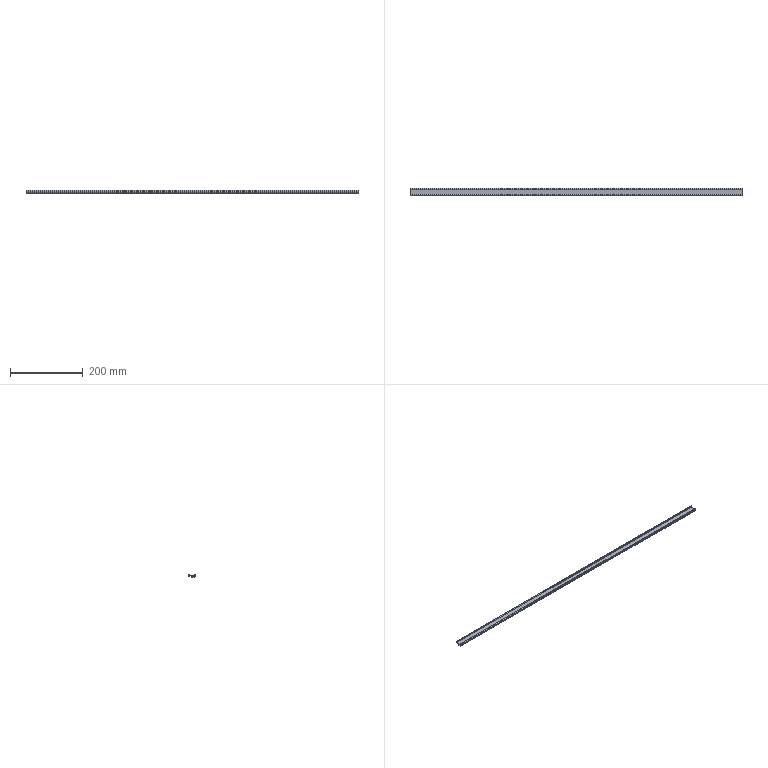Part | SolidWorks | features Extrusion 1 | 1 solid | 37 faces | box 915 x 19.991 x 9 mm | volume 36941 mm3 | cylinder 19 | plane 18 | commonest cylinder face diameters 2 x6 0.5 x5 0.2 x2 3 x2 4.958 x2 3.038 x1
STEP:
#1=CARTESIAN_POINT('',(492.5,771.135,454.913));
#2=VERTEX_POINT('',#1);
#3=CARTESIAN_POINT('',(492.5,769.976,455.201));
#4=VERTEX_POINT('',#3);
#5=CARTESIAN_POINT('',(492.5,769.976,452.722));
#6=DIRECTION('',(1.,0.,0.));
#7=DIRECTION('',(0.,0.,-1.));
#8=AXIS2_PLACEMENT_3D('',#5,#6,#7);
#9=CIRCLE('',#8,2.479);
#10=EDGE_CURVE('',#2,#4,#9,.T.);
#11=ORIENTED_EDGE('',*,*,#10,.T.);
#12=CARTESIAN_POINT('',(-422.5,769.976,455.201));
#13=VERTEX_POINT('',#12);
#14=CARTESIAN_POINT('',(492.5,769.976,455.201));
#15=DIRECTION('',(-1.,0.,0.));
#16=VECTOR('',#15,1000.);
#17=LINE('',#14,#16);
#18=EDGE_CURVE('',#4,#13,#17,.T.);
#19=ORIENTED_EDGE('',*,*,#18,.T.);
#20=CARTESIAN_POINT('',(-422.5,771.135,454.913));
#21=VERTEX_POINT('',#20);
#22=CARTESIAN_POINT('',(-422.5,769.976,452.722));
#23=DIRECTION('',(1.,0.,0.));
#24=DIRECTION('',(0.,0.,-1.));
#25=AXIS2_PLACEMENT_3D('',#22,#23,#24);
#26=CIRCLE('',#25,2.479);
#27=EDGE_CURVE('',#21,#13,#26,.T.);
#28=ORIENTED_EDGE('',*,*,#27,.F.);
#29=CARTESIAN_POINT('',(492.5,771.135,454.913));
#30=DIRECTION('',(-1.,0.,0.));
#31=VECTOR('',#30,1000.);
#32=LINE('',#29,#31);
#33=EDGE_CURVE('',#2,#21,#32,.T.);
#34=ORIENTED_EDGE('',*,*,#33,.F.);
#35=EDGE_LOOP('',(#11,#19,#28,#34));
#36=FACE_OUTER_BOUND('',#35,.T.);
#37=CARTESIAN_POINT('',(492.5,769.976,452.722));
#38=DIRECTION('',(-1.,0.,0.));
#39=DIRECTION('',(0.,0.,1.));
#40=AXIS2_PLACEMENT_3D('',#37,#38,#39);
#41=CYLINDRICAL_SURFACE('',#40,2.479);
#42=ADVANCED_FACE('',(#36),#41,.F.);
#43=CARTESIAN_POINT('',(-422.5,755.36,455.2));
#44=VERTEX_POINT('',#43);
#45=CARTESIAN_POINT('',(-422.5,755.11,454.95));
#46=VERTEX_POINT('',#45);
#47=CARTESIAN_POINT('',(-422.5,755.36,454.95));
#48=DIRECTION('',(1.,0.,0.));
#49=DIRECTION('',(0.,0.,-1.));
#50=AXIS2_PLACEMENT_3D('',#47,#48,#49);
#51=CIRCLE('',#50,0.25);
#52=EDGE_CURVE('',#44,#46,#51,.T.);
#53=ORIENTED_EDGE('',*,*,#52,.F.);
#54=CARTESIAN_POINT('',(492.5,755.36,455.2));
#55=VERTEX_POINT('',#54);
#56=CARTESIAN_POINT('',(492.5,755.36,455.2));
#57=DIRECTION('',(-1.,0.,0.));
#58=VECTOR('',#57,1000.);
#59=LINE('',#56,#58);
#60=EDGE_CURVE('',#55,#44,#59,.T.);
#61=ORIENTED_EDGE('',*,*,#60,.F.);
#62=CARTESIAN_POINT('',(492.5,755.11,454.95));
#63=VERTEX_POINT('',#62);
#64=CARTESIAN_POINT('',(492.5,755.36,454.95));
#65=DIRECTION('',(1.,0.,0.));
#66=DIRECTION('',(0.,0.,-1.));
#67=AXIS2_PLACEMENT_3D('',#64,#65,#66);
#68=CIRCLE('',#67,0.25);
#69=EDGE_CURVE('',#55,#63,#68,.T.);
#70=ORIENTED_EDGE('',*,*,#69,.T.);
#71=CARTESIAN_POINT('',(492.5,755.11,454.95));
#72=DIRECTION('',(-1.,0.,0.));
#73=VECTOR('',#72,1000.);
#74=LINE('',#71,#73);
#75=EDGE_CURVE('',#63,#46,#74,.T.);
#76=ORIENTED_EDGE('',*,*,#75,.T.);
#77=EDGE_LOOP('',(#53,#61,#70,#76));
#78=FACE_OUTER_BOUND('',#77,.T.);
#79=CARTESIAN_POINT('',(492.5,755.36,454.95));
#80=DIRECTION('',(-1.,0.,0.));
#81=DIRECTION('',(0.,0.,1.));
#82=AXIS2_PLACEMENT_3D('',#79,#80,#81);
#83=CYLINDRICAL_SURFACE('',#82,0.25);
#84=ADVANCED_FACE('',(#78),#83,.F.);
#85=CARTESIAN_POINT('',(-422.5,769.91,455.2));
#86=VERTEX_POINT('',#85);
#87=CARTESIAN_POINT('',(-422.5,769.91,455.2));
#88=DIRECTION('',(0.,-1.,0.));
#89=VECTOR('',#88,1000.);
#90=LINE('',#87,#89);
#91=EDGE_CURVE('',#86,#44,#90,.T.);
#92=ORIENTED_EDGE('',*,*,#91,.F.);
#93=CARTESIAN_POINT('',(492.5,769.91,455.2));
#94=VERTEX_POINT('',#93);
#95=CARTESIAN_POINT('',(492.5,769.91,455.2));
#96=DIRECTION('',(-1.,0.,0.));
#97=VECTOR('',#96,1000.);
#98=LINE('',#95,#97);
#99=EDGE_CURVE('',#94,#86,#98,.T.);
#100=ORIENTED_EDGE('',*,*,#99,.F.);
#101=CARTESIAN_POINT('',(492.5,769.91,455.2));
#102=DIRECTION('',(0.,-1.,0.));
#103=VECTOR('',#102,1000.);
#104=LINE('',#101,#103);
#105=EDGE_CURVE('',#94,#55,#104,.T.);
#106=ORIENTED_EDGE('',*,*,#105,.T.);
#107=ORIENTED_EDGE('',*,*,#60,.T.);
#108=EDGE_LOOP('',(#92,#100,#106,#107));
#109=FACE_OUTER_BOUND('',#108,.T.);
#110=CARTESIAN_POINT('',(492.5,769.91,455.2));
#111=DIRECTION('',(0.,0.,-1.));
#112=DIRECTION('',(0.,1.,0.));
#113=AXIS2_PLACEMENT_3D('',#110,#111,#112);
#114=PLANE('',#113);
#115=ADVANCED_FACE('',(#109),#114,.T.);
#116=ORIENTED_EDGE('',*,*,#18,.F.);
#117=CARTESIAN_POINT('',(492.5,769.976,452.722));
#118=DIRECTION('',(1.,0.,0.));
#119=DIRECTION('',(0.,0.,-1.));
#120=AXIS2_PLACEMENT_3D('',#117,#118,#119);
#121=CIRCLE('',#120,2.479);
#122=EDGE_CURVE('',#4,#94,#121,.T.);
#123=ORIENTED_EDGE('',*,*,#122,.T.);
#124=ORIENTED_EDGE('',*,*,#99,.T.);
#125=CARTESIAN_POINT('',(-422.5,769.976,452.722));
#126=DIRECTION('',(1.,0.,0.));
#127=DIRECTION('',(0.,0.,-1.));
#128=AXIS2_PLACEMENT_3D('',#125,#126,#127);
#129=CIRCLE('',#128,2.479);
#130=EDGE_CURVE('',#13,#86,#129,.T.);
#131=ORIENTED_EDGE('',*,*,#130,.F.);
#132=EDGE_LOOP('',(#116,#123,#124,#131));
#133=FACE_OUTER_BOUND('',#132,.T.);
#134=CARTESIAN_POINT('',(492.5,769.976,452.722));
#135=DIRECTION('',(-1.,0.,0.));
#136=DIRECTION('',(0.,0.,1.));
#137=AXIS2_PLACEMENT_3D('',#134,#135,#136);
#138=CYLINDRICAL_SURFACE('',#137,2.479);
#139=ADVANCED_FACE('',(#133),#138,.F.);
#140=CARTESIAN_POINT('',(-422.5,771.197,454.903));
#141=VERTEX_POINT('',#140);
#142=CARTESIAN_POINT('',(-422.5,771.182,455.002));
#143=DIRECTION('',(-1.,0.,0.));
#144=DIRECTION('',(0.,0.,1.));
#145=AXIS2_PLACEMENT_3D('',#142,#143,#144);
#146=CIRCLE('',#145,0.1);
#147=EDGE_CURVE('',#141,#21,#146,.T.);
#148=ORIENTED_EDGE('',*,*,#147,.F.);
#149=CARTESIAN_POINT('',(492.5,771.197,454.903));
#150=VERTEX_POINT('',#149);
#151=CARTESIAN_POINT('',(492.5,771.197,454.903));
#152=DIRECTION('',(-1.,0.,0.));
#153=VECTOR('',#152,1000.);
#154=LINE('',#151,#153);
#155=EDGE_CURVE('',#150,#141,#154,.T.);
#156=ORIENTED_EDGE('',*,*,#155,.F.);
#157=CARTESIAN_POINT('',(492.5,771.182,455.002));
#158=DIRECTION('',(-1.,0.,0.));
#159=DIRECTION('',(0.,0.,1.));
#160=AXIS2_PLACEMENT_3D('',#157,#158,#159);
#161=CIRCLE('',#160,0.1);
#162=EDGE_CURVE('',#150,#2,#161,.T.);
#163=ORIENTED_EDGE('',*,*,#162,.T.);
#164=ORIENTED_EDGE('',*,*,#33,.T.);
#165=EDGE_LOOP('',(#148,#156,#163,#164));
#166=FACE_OUTER_BOUND('',#165,.T.);
#167=CARTESIAN_POINT('',(492.5,771.182,455.002));
#168=DIRECTION('',(-1.,0.,0.));
#169=DIRECTION('',(0.,0.,1.));
#170=AXIS2_PLACEMENT_3D('',#167,#168,#169);
#171=CYLINDRICAL_SURFACE('',#170,0.1);
#172=ADVANCED_FACE('',(#166),#171,.T.);
#173=CARTESIAN_POINT('',(-422.5,771.395,455.064));
#174=VERTEX_POINT('',#173);
#175=CARTESIAN_POINT('',(-422.5,771.16,455.15));
#176=DIRECTION('',(-1.,0.,0.));
#177=DIRECTION('',(0.,0.,1.));
#178=AXIS2_PLACEMENT_3D('',#175,#176,#177);
#179=CIRCLE('',#178,0.25);
#180=EDGE_CURVE('',#174,#141,#179,.T.);
#181=ORIENTED_EDGE('',*,*,#180,.F.);
#182=CARTESIAN_POINT('',(492.5,771.395,455.064));
#183=VERTEX_POINT('',#182);
#184=CARTESIAN_POINT('',(492.5,771.395,455.064));
#185=DIRECTION('',(-1.,0.,0.));
#186=VECTOR('',#185,1000.);
#187=LINE('',#184,#186);
#188=EDGE_CURVE('',#183,#174,#187,.T.);
#189=ORIENTED_EDGE('',*,*,#188,.F.);
#190=CARTESIAN_POINT('',(492.5,771.16,455.15));
#191=DIRECTION('',(-1.,0.,0.));
#192=DIRECTION('',(0.,0.,1.));
#193=AXIS2_PLACEMENT_3D('',#190,#191,#192);
#194=CIRCLE('',#193,0.25);
#195=EDGE_CURVE('',#183,#150,#194,.T.);
#196=ORIENTED_EDGE('',*,*,#195,.T.);
#197=ORIENTED_EDGE('',*,*,#155,.T.);
#198=EDGE_LOOP('',(#181,#189,#196,#197));
#199=FACE_OUTER_BOUND('',#198,.T.);
#200=CARTESIAN_POINT('',(492.5,771.16,455.15));
#201=DIRECTION('',(-1.,0.,0.));
#202=DIRECTION('',(0.,0.,1.));
#203=AXIS2_PLACEMENT_3D('',#200,#201,#202);
#204=CYLINDRICAL_SURFACE('',#203,0.25);
#205=ADVANCED_FACE('',(#199),#204,.T.);
#206=CARTESIAN_POINT('',(-422.5,771.353,455.183));
#207=VERTEX_POINT('',#206);
#208=CARTESIAN_POINT('',(-422.5,771.301,455.098));
#209=DIRECTION('',(-1.,0.,0.));
#210=DIRECTION('',(0.,0.,1.));
#211=AXIS2_PLACEMENT_3D('',#208,#209,#210);
#212=CIRCLE('',#211,0.1);
#213=EDGE_CURVE('',#207,#174,#212,.T.);
#214=ORIENTED_EDGE('',*,*,#213,.F.);
#215=CARTESIAN_POINT('',(492.5,771.353,455.183));
#216=VERTEX_POINT('',#215);
#217=CARTESIAN_POINT('',(492.5,771.353,455.183));
#218=DIRECTION('',(-1.,0.,0.));
#219=VECTOR('',#218,1000.);
#220=LINE('',#217,#219);
#221=EDGE_CURVE('',#216,#207,#220,.T.);
#222=ORIENTED_EDGE('',*,*,#221,.F.);
#223=CARTESIAN_POINT('',(492.5,771.301,455.098));
#224=DIRECTION('',(-1.,0.,0.));
#225=DIRECTION('',(0.,0.,1.));
#226=AXIS2_PLACEMENT_3D('',#223,#224,#225);
#227=CIRCLE('',#226,0.1);
#228=EDGE_CURVE('',#216,#183,#227,.T.);
#229=ORIENTED_EDGE('',*,*,#228,.T.);
#230=ORIENTED_EDGE('',*,*,#188,.T.);
#231=EDGE_LOOP('',(#214,#222,#229,#230));
#232=FACE_OUTER_BOUND('',#231,.T.);
#233=CARTESIAN_POINT('',(492.5,771.301,455.098));
#234=DIRECTION('',(-1.,0.,0.));
#235=DIRECTION('',(0.,0.,1.));
#236=AXIS2_PLACEMENT_3D('',#233,#234,#235);
#237=CYLINDRICAL_SURFACE('',#236,0.1);
#238=ADVANCED_FACE('',(#232),#237,.T.);
#239=CARTESIAN_POINT('',(-422.5,770.71,456.));
#240=VERTEX_POINT('',#239);
#241=CARTESIAN_POINT('',(-422.5,772.153,456.475));
#242=DIRECTION('',(1.,0.,0.));
#243=DIRECTION('',(0.,0.,-1.));
#244=AXIS2_PLACEMENT_3D('',#241,#242,#243);
#245=CIRCLE('',#244,1.519);
#246=EDGE_CURVE('',#240,#207,#245,.T.);
#247=ORIENTED_EDGE('',*,*,#246,.F.);
#248=CARTESIAN_POINT('',(492.5,770.71,456.));
#249=VERTEX_POINT('',#248);
#250=CARTESIAN_POINT('',(492.5,770.71,456.));
#251=DIRECTION('',(-1.,0.,0.));
#252=VECTOR('',#251,1000.);
#253=LINE('',#250,#252);
#254=EDGE_CURVE('',#249,#240,#253,.T.);
#255=ORIENTED_EDGE('',*,*,#254,.F.);
#256=CARTESIAN_POINT('',(492.5,772.153,456.475));
#257=DIRECTION('',(1.,0.,0.));
#258=DIRECTION('',(0.,0.,-1.));
#259=AXIS2_PLACEMENT_3D('',#256,#257,#258);
#260=CIRCLE('',#259,1.519);
#261=EDGE_CURVE('',#249,#216,#260,.T.);
#262=ORIENTED_EDGE('',*,*,#261,.T.);
#263=ORIENTED_EDGE('',*,*,#221,.T.);
#264=EDGE_LOOP('',(#247,#255,#262,#263));
#265=FACE_OUTER_BOUND('',#264,.T.);
#266=CARTESIAN_POINT('',(492.5,772.153,456.475));
#267=DIRECTION('',(-1.,0.,0.));
#268=DIRECTION('',(0.,0.,1.));
#269=AXIS2_PLACEMENT_3D('',#266,#267,#268);
#270=CYLINDRICAL_SURFACE('',#269,1.519);
#271=ADVANCED_FACE('',(#265),#270,.F.);
#272=CARTESIAN_POINT('',(-422.5,770.71,458.6));
#273=VERTEX_POINT('',#272);
#274=CARTESIAN_POINT('',(-422.5,770.71,458.6));
#275=DIRECTION('',(0.,0.,-1.));
#276=VECTOR('',#275,1000.);
#277=LINE('',#274,#276);
#278=EDGE_CURVE('',#273,#240,#277,.T.);
#279=ORIENTED_EDGE('',*,*,#278,.F.);
#280=CARTESIAN_POINT('',(492.5,770.71,458.6));
#281=VERTEX_POINT('',#280);
#282=CARTESIAN_POINT('',(492.5,770.71,458.6));
#283=DIRECTION('',(-1.,0.,0.));
#284=VECTOR('',#283,1000.);
#285=LINE('',#282,#284);
#286=EDGE_CURVE('',#281,#273,#285,.T.);
#287=ORIENTED_EDGE('',*,*,#286,.F.);
#288=CARTESIAN_POINT('',(492.5,770.71,458.6));
#289=DIRECTION('',(0.,0.,-1.));
#290=VECTOR('',#289,1000.);
#291=LINE('',#288,#290);
#292=EDGE_CURVE('',#281,#249,#291,.T.);
#293=ORIENTED_EDGE('',*,*,#292,.T.);
#294=ORIENTED_EDGE('',*,*,#254,.T.);
#295=EDGE_LOOP('',(#279,#287,#293,#294));
#296=FACE_OUTER_BOUND('',#295,.T.);
#297=CARTESIAN_POINT('',(492.5,770.71,458.6));
#298=DIRECTION('',(0.,1.,0.));
#299=DIRECTION('',(-1.,0.,0.));
#300=AXIS2_PLACEMENT_3D('',#297,#298,#299);
#301=PLANE('',#300);
#302=ADVANCED_FACE('',(#296),#301,.T.);
#303=CARTESIAN_POINT('',(-422.5,769.21,460.1));
#304=VERTEX_POINT('',#303);
#305=CARTESIAN_POINT('',(-422.5,769.21,458.6));
#306=DIRECTION('',(-1.,0.,0.));
#307=DIRECTION('',(0.,0.,1.));
#308=AXIS2_PLACEMENT_3D('',#305,#306,#307);
#309=CIRCLE('',#308,1.5);
#310=EDGE_CURVE('',#304,#273,#309,.T.);
#311=ORIENTED_EDGE('',*,*,#310,.F.);
#312=CARTESIAN_POINT('',(492.5,769.21,460.1));
#313=VERTEX_POINT('',#312);
#314=CARTESIAN_POINT('',(492.5,769.21,460.1));
#315=DIRECTION('',(-1.,0.,0.));
#316=VECTOR('',#315,1000.);
#317=LINE('',#314,#316);
#318=EDGE_CURVE('',#313,#304,#317,.T.);
#319=ORIENTED_EDGE('',*,*,#318,.F.);
#320=CARTESIAN_POINT('',(492.5,769.21,458.6));
#321=DIRECTION('',(-1.,0.,0.));
#322=DIRECTION('',(0.,0.,1.));
#323=AXIS2_PLACEMENT_3D('',#320,#321,#322);
#324=CIRCLE('',#323,1.5);
#325=EDGE_CURVE('',#313,#281,#324,.T.);
#326=ORIENTED_EDGE('',*,*,#325,.T.);
#327=ORIENTED_EDGE('',*,*,#286,.T.);
#328=EDGE_LOOP('',(#311,#319,#326,#327));
#329=FACE_OUTER_BOUND('',#328,.T.);
#330=CARTESIAN_POINT('',(492.5,769.21,458.6));
#331=DIRECTION('',(-1.,0.,0.));
#332=DIRECTION('',(0.,0.,1.));
#333=AXIS2_PLACEMENT_3D('',#330,#331,#332);
#334=CYLINDRICAL_SURFACE('',#333,1.5);
#335=ADVANCED_FACE('',(#329),#334,.T.);
#336=CARTESIAN_POINT('',(-422.5,768.81,460.1));
#337=VERTEX_POINT('',#336);
#338=CARTESIAN_POINT('',(-422.5,768.81,460.1));
#339=DIRECTION('',(0.,1.,0.));
#340=VECTOR('',#339,1000.);
#341=LINE('',#338,#340);
#342=EDGE_CURVE('',#337,#304,#341,.T.);
#343=ORIENTED_EDGE('',*,*,#342,.F.);
#344=CARTESIAN_POINT('',(492.5,768.81,460.1));
#345=VERTEX_POINT('',#344);
#346=CARTESIAN_POINT('',(492.5,768.81,460.1));
#347=DIRECTION('',(-1.,0.,0.));
#348=VECTOR('',#347,1000.);
#349=LINE('',#346,#348);
#350=EDGE_CURVE('',#345,#337,#349,.T.);
#351=ORIENTED_EDGE('',*,*,#350,.F.);
#352=CARTESIAN_POINT('',(492.5,768.81,460.1));
#353=DIRECTION('',(0.,1.,0.));
#354=VECTOR('',#353,1000.);
#355=LINE('',#352,#354);
#356=EDGE_CURVE('',#345,#313,#355,.T.);
#357=ORIENTED_EDGE('',*,*,#356,.T.);
#358=ORIENTED_EDGE('',*,*,#318,.T.);
#359=EDGE_LOOP('',(#343,#351,#357,#358));
#360=FACE_OUTER_BOUND('',#359,.T.);
#361=CARTESIAN_POINT('',(492.5,768.81,460.1));
#362=DIRECTION('',(0.,0.,1.));
#363=DIRECTION('',(1.,0.,0.));
#364=AXIS2_PLACEMENT_3D('',#361,#362,#363);
#365=PLANE('',#364);
#366=ADVANCED_FACE('',(#360),#365,.T.);
#367=CARTESIAN_POINT('',(-422.5,768.547,458.135));
#368=VERTEX_POINT('',#367);
#369=CARTESIAN_POINT('',(-422.5,768.81,459.1));
#370=DIRECTION('',(-1.,0.,0.));
#371=DIRECTION('',(0.,0.,1.));
#372=AXIS2_PLACEMENT_3D('',#369,#370,#371);
#373=CIRCLE('',#372,1.);
#374=EDGE_CURVE('',#368,#337,#373,.T.);
#375=ORIENTED_EDGE('',*,*,#374,.F.);
#376=CARTESIAN_POINT('',(492.5,768.547,458.135));
#377=VERTEX_POINT('',#376);
#378=CARTESIAN_POINT('',(492.5,768.547,458.135));
#379=DIRECTION('',(-1.,0.,0.));
#380=VECTOR('',#379,1000.);
#381=LINE('',#378,#380);
#382=EDGE_CURVE('',#377,#368,#381,.T.);
#383=ORIENTED_EDGE('',*,*,#382,.F.);
#384=CARTESIAN_POINT('',(492.5,768.81,459.1));
#385=DIRECTION('',(-1.,0.,0.));
#386=DIRECTION('',(0.,0.,1.));
#387=AXIS2_PLACEMENT_3D('',#384,#385,#386);
#388=CIRCLE('',#387,1.);
#389=EDGE_CURVE('',#377,#345,#388,.T.);
#390=ORIENTED_EDGE('',*,*,#389,.T.);
#391=ORIENTED_EDGE('',*,*,#350,.T.);
#392=EDGE_LOOP('',(#375,#383,#390,#391));
#393=FACE_OUTER_BOUND('',#392,.T.);
#394=CARTESIAN_POINT('',(492.5,768.81,459.1));
#395=DIRECTION('',(-1.,0.,0.));
#396=DIRECTION('',(0.,0.,1.));
#397=AXIS2_PLACEMENT_3D('',#394,#395,#396);
#398=CYLINDRICAL_SURFACE('',#397,1.);
#399=ADVANCED_FACE('',(#393),#398,.T.);
#400=CARTESIAN_POINT('',(-422.5,769.173,457.965));
#401=VERTEX_POINT('',#400);
#402=CARTESIAN_POINT('',(-422.5,769.173,457.965));
#403=DIRECTION('',(0.,-0.9649,0.2627));
#404=VECTOR('',#403,1000.);
#405=LINE('',#402,#404);
#406=EDGE_CURVE('',#401,#368,#405,.T.);
#407=ORIENTED_EDGE('',*,*,#406,.F.);
#408=CARTESIAN_POINT('',(492.5,769.173,457.965));
#409=VERTEX_POINT('',#408);
#410=CARTESIAN_POINT('',(492.5,769.173,457.965));
#411=DIRECTION('',(-1.,0.,0.));
#412=VECTOR('',#411,1000.);
#413=LINE('',#410,#412);
#414=EDGE_CURVE('',#409,#401,#413,.T.);
#415=ORIENTED_EDGE('',*,*,#414,.F.);
#416=CARTESIAN_POINT('',(492.5,769.173,457.965));
#417=DIRECTION('',(0.,-0.9649,0.2627));
#418=VECTOR('',#417,1000.);
#419=LINE('',#416,#418);
#420=EDGE_CURVE('',#409,#377,#419,.T.);
#421=ORIENTED_EDGE('',*,*,#420,.T.);
#422=ORIENTED_EDGE('',*,*,#382,.T.);
#423=EDGE_LOOP('',(#407,#415,#421,#422));
#424=FACE_OUTER_BOUND('',#423,.T.);
#425=CARTESIAN_POINT('',(492.5,769.173,457.965));
#426=DIRECTION('',(0.,-0.2627,-0.9649));
#427=DIRECTION('',(0.,0.9649,-0.2627));
#428=AXIS2_PLACEMENT_3D('',#425,#426,#427);
#429=PLANE('',#428);
#430=ADVANCED_FACE('',(#424),#429,.T.);
#431=CARTESIAN_POINT('',(-422.5,768.91,456.));
#432=VERTEX_POINT('',#431);
#433=CARTESIAN_POINT('',(-422.5,768.91,457.));
#434=DIRECTION('',(1.,0.,0.));
#435=DIRECTION('',(0.,0.,-1.));
#436=AXIS2_PLACEMENT_3D('',#433,#434,#435);
#437=CIRCLE('',#436,1.);
#438=EDGE_CURVE('',#432,#401,#437,.T.);
#439=ORIENTED_EDGE('',*,*,#438,.F.);
#440=CARTESIAN_POINT('',(492.5,768.91,456.));
#441=VERTEX_POINT('',#440);
#442=CARTESIAN_POINT('',(492.5,768.91,456.));
#443=DIRECTION('',(-1.,0.,0.));
#444=VECTOR('',#443,1000.);
#445=LINE('',#442,#444);
#446=EDGE_CURVE('',#441,#432,#445,.T.);
#447=ORIENTED_EDGE('',*,*,#446,.F.);
#448=CARTESIAN_POINT('',(492.5,768.91,457.));
#449=DIRECTION('',(1.,0.,0.));
#450=DIRECTION('',(0.,0.,-1.));
#451=AXIS2_PLACEMENT_3D('',#448,#449,#450);
#452=CIRCLE('',#451,1.);
#453=EDGE_CURVE('',#441,#409,#452,.T.);
#454=ORIENTED_EDGE('',*,*,#453,.T.);
#455=ORIENTED_EDGE('',*,*,#414,.T.);
#456=EDGE_LOOP('',(#439,#447,#454,#455));
#457=FACE_OUTER_BOUND('',#456,.T.);
#458=CARTESIAN_POINT('',(492.5,768.91,457.));
#459=DIRECTION('',(-1.,0.,0.));
#460=DIRECTION('',(0.,0.,1.));
#461=AXIS2_PLACEMENT_3D('',#458,#459,#460);
#462=CYLINDRICAL_SURFACE('',#461,1.);
#463=ADVANCED_FACE('',(#457),#462,.F.);
#464=CARTESIAN_POINT('',(-422.5,753.21,456.));
#465=VERTEX_POINT('',#464);
#466=CARTESIAN_POINT('',(-422.5,753.21,456.));
#467=DIRECTION('',(0.,1.,0.));
#468=VECTOR('',#467,1000.);
#469=LINE('',#466,#468);
#470=EDGE_CURVE('',#465,#432,#469,.T.);
#471=ORIENTED_EDGE('',*,*,#470,.F.);
#472=CARTESIAN_POINT('',(492.5,753.21,456.));
#473=VERTEX_POINT('',#472);
#474=CARTESIAN_POINT('',(492.5,753.21,456.));
#475=DIRECTION('',(-1.,0.,0.));
#476=VECTOR('',#475,1000.);
#477=LINE('',#474,#476);
#478=EDGE_CURVE('',#473,#465,#477,.T.);
#479=ORIENTED_EDGE('',*,*,#478,.F.);
#480=CARTESIAN_POINT('',(492.5,753.21,456.));
#481=DIRECTION('',(0.,1.,0.));
#482=VECTOR('',#481,1000.);
#483=LINE('',#480,#482);
#484=EDGE_CURVE('',#473,#441,#483,.T.);
#485=ORIENTED_EDGE('',*,*,#484,.T.);
#486=ORIENTED_EDGE('',*,*,#446,.T.);
#487=EDGE_LOOP('',(#471,#479,#485,#486));
#488=FACE_OUTER_BOUND('',#487,.T.);
#489=CARTESIAN_POINT('',(492.5,753.21,456.));
#490=DIRECTION('',(0.,0.,1.));
#491=DIRECTION('',(0.,-1.,0.));
#492=AXIS2_PLACEMENT_3D('',#489,#490,#491);
#493=PLANE('',#492);
#494=ADVANCED_FACE('',(#488),#493,.T.);
#495=CARTESIAN_POINT('',(-422.5,752.947,457.965));
#496=VERTEX_POINT('',#495);
#497=CARTESIAN_POINT('',(-422.5,753.21,457.));
#498=DIRECTION('',(1.,0.,0.));
#499=DIRECTION('',(0.,0.,-1.));
#500=AXIS2_PLACEMENT_3D('',#497,#498,#499);
#501=CIRCLE('',#500,1.);
#502=EDGE_CURVE('',#496,#465,#501,.T.);
#503=ORIENTED_EDGE('',*,*,#502,.F.);
#504=CARTESIAN_POINT('',(492.5,752.947,457.965));
#505=VERTEX_POINT('',#504);
#506=CARTESIAN_POINT('',(492.5,752.947,457.965));
#507=DIRECTION('',(-1.,0.,0.));
#508=VECTOR('',#507,1000.);
#509=LINE('',#506,#508);
#510=EDGE_CURVE('',#505,#496,#509,.T.);
#511=ORIENTED_EDGE('',*,*,#510,.F.);
#512=CARTESIAN_POINT('',(492.5,753.21,457.));
#513=DIRECTION('',(1.,0.,0.));
#514=DIRECTION('',(0.,0.,-1.));
#515=AXIS2_PLACEMENT_3D('',#512,#513,#514);
#516=CIRCLE('',#515,1.);
#517=EDGE_CURVE('',#505,#473,#516,.T.);
#518=ORIENTED_EDGE('',*,*,#517,.T.);
#519=ORIENTED_EDGE('',*,*,#478,.T.);
#520=EDGE_LOOP('',(#503,#511,#518,#519));
#521=FACE_OUTER_BOUND('',#520,.T.);
#522=CARTESIAN_POINT('',(492.5,753.21,457.));
#523=DIRECTION('',(-1.,0.,0.));
#524=DIRECTION('',(0.,0.,1.));
#525=AXIS2_PLACEMENT_3D('',#522,#523,#524);
#526=CYLINDRICAL_SURFACE('',#525,1.);
#527=ADVANCED_FACE('',(#521),#526,.F.);
#528=CARTESIAN_POINT('',(-422.5,753.573,458.135));
#529=VERTEX_POINT('',#528);
#530=CARTESIAN_POINT('',(-422.5,753.573,458.135));
#531=DIRECTION('',(0.,-0.9649,-0.2627));
#532=VECTOR('',#531,1000.);
#533=LINE('',#530,#532);
#534=EDGE_CURVE('',#529,#496,#533,.T.);
#535=ORIENTED_EDGE('',*,*,#534,.F.);
#536=CARTESIAN_POINT('',(492.5,753.573,458.135));
#537=VERTEX_POINT('',#536);
#538=CARTESIAN_POINT('',(492.5,753.573,458.135));
#539=DIRECTION('',(-1.,0.,0.));
#540=VECTOR('',#539,1000.);
#541=LINE('',#538,#540);
#542=EDGE_CURVE('',#537,#529,#541,.T.);
#543=ORIENTED_EDGE('',*,*,#542,.F.);
#544=CARTESIAN_POINT('',(492.5,753.573,458.135));
#545=DIRECTION('',(0.,-0.9649,-0.2627));
#546=VECTOR('',#545,1000.);
#547=LINE('',#544,#546);
#548=EDGE_CURVE('',#537,#505,#547,.T.);
#549=ORIENTED_EDGE('',*,*,#548,.T.);
#550=ORIENTED_EDGE('',*,*,#510,.T.);
#551=EDGE_LOOP('',(#535,#543,#549,#550));
#552=FACE_OUTER_BOUND('',#551,.T.);
#553=CARTESIAN_POINT('',(492.5,753.573,458.135));
#554=DIRECTION('',(0.,0.2627,-0.9649));
#555=DIRECTION('',(0.,0.9649,0.2627));
#556=AXIS2_PLACEMENT_3D('',#553,#554,#555);
#557=PLANE('',#556);
#558=ADVANCED_FACE('',(#552),#557,.T.);
#559=CARTESIAN_POINT('',(-422.5,753.31,460.1));
#560=VERTEX_POINT('',#559);
#561=CARTESIAN_POINT('',(-422.5,753.31,459.1));
#562=DIRECTION('',(-1.,0.,0.));
#563=DIRECTION('',(0.,0.,1.));
#564=AXIS2_PLACEMENT_3D('',#561,#562,#563);
#565=CIRCLE('',#564,1.);
#566=EDGE_CURVE('',#560,#529,#565,.T.);
#567=ORIENTED_EDGE('',*,*,#566,.F.);
#568=CARTESIAN_POINT('',(492.5,753.31,460.1));
#569=VERTEX_POINT('',#568);
#570=CARTESIAN_POINT('',(492.5,753.31,460.1));
#571=DIRECTION('',(-1.,0.,0.));
#572=VECTOR('',#571,1000.);
#573=LINE('',#570,#572);
#574=EDGE_CURVE('',#569,#560,#573,.T.);
#575=ORIENTED_EDGE('',*,*,#574,.F.);
#576=CARTESIAN_POINT('',(492.5,753.31,459.1));
#577=DIRECTION('',(-1.,0.,0.));
#578=DIRECTION('',(0.,0.,1.));
#579=AXIS2_PLACEMENT_3D('',#576,#577,#578);
#580=CIRCLE('',#579,1.);
#581=EDGE_CURVE('',#569,#537,#580,.T.);
#582=ORIENTED_EDGE('',*,*,#581,.T.);
#583=ORIENTED_EDGE('',*,*,#542,.T.);
#584=EDGE_LOOP('',(#567,#575,#582,#583));
#585=FACE_OUTER_BOUND('',#584,.T.);
#586=CARTESIAN_POINT('',(492.5,753.31,459.1));
#587=DIRECTION('',(-1.,0.,0.));
#588=DIRECTION('',(0.,0.,1.));
#589=AXIS2_PLACEMENT_3D('',#586,#587,#588);
#590=CYLINDRICAL_SURFACE('',#589,1.);
#591=ADVANCED_FACE('',(#585),#590,.T.);
#592=CARTESIAN_POINT('',(-422.5,752.91,460.1));
#593=VERTEX_POINT('',#592);
#594=CARTESIAN_POINT('',(-422.5,752.91,460.1));
#595=DIRECTION('',(0.,1.,0.));
#596=VECTOR('',#595,1000.);
#597=LINE('',#594,#596);
#598=EDGE_CURVE('',#593,#560,#597,.T.);
#599=ORIENTED_EDGE('',*,*,#598,.F.);
#600=CARTESIAN_POINT('',(492.5,752.91,460.1));
#601=VERTEX_POINT('',#600);
#602=CARTESIAN_POINT('',(492.5,752.91,460.1));
#603=DIRECTION('',(-1.,0.,0.));
#604=VECTOR('',#603,1000.);
#605=LINE('',#602,#604);
#606=EDGE_CURVE('',#601,#593,#605,.T.);
#607=ORIENTED_EDGE('',*,*,#606,.F.);
#608=CARTESIAN_POINT('',(492.5,752.91,460.1));
#609=DIRECTION('',(0.,1.,0.));
#610=VECTOR('',#609,1000.);
#611=LINE('',#608,#610);
#612=EDGE_CURVE('',#601,#569,#611,.T.);
#613=ORIENTED_EDGE('',*,*,#612,.T.);
#614=ORIENTED_EDGE('',*,*,#574,.T.);
#615=EDGE_LOOP('',(#599,#607,#613,#614));
#616=FACE_OUTER_BOUND('',#615,.T.);
#617=CARTESIAN_POINT('',(492.5,752.91,460.1));
#618=DIRECTION('',(0.,0.,1.));
#619=DIRECTION('',(1.,0.,0.));
#620=AXIS2_PLACEMENT_3D('',#617,#618,#619);
#621=PLANE('',#620);
#622=ADVANCED_FACE('',(#616),#621,.T.);
#623=CARTESIAN_POINT('',(-422.5,751.41,458.6));
#624=VERTEX_POINT('',#623);
#625=CARTESIAN_POINT('',(-422.5,752.91,458.6));
#626=DIRECTION('',(-1.,0.,0.));
#627=DIRECTION('',(0.,0.,1.));
#628=AXIS2_PLACEMENT_3D('',#625,#626,#627);
#629=CIRCLE('',#628,1.5);
#630=EDGE_CURVE('',#624,#593,#629,.T.);
#631=ORIENTED_EDGE('',*,*,#630,.F.);
#632=CARTESIAN_POINT('',(492.5,751.41,458.6));
#633=VERTEX_POINT('',#632);
#634=CARTESIAN_POINT('',(492.5,751.41,458.6));
#635=DIRECTION('',(-1.,0.,0.));
#636=VECTOR('',#635,1000.);
#637=LINE('',#634,#636);
#638=EDGE_CURVE('',#633,#624,#637,.T.);
#639=ORIENTED_EDGE('',*,*,#638,.F.);
#640=CARTESIAN_POINT('',(492.5,752.91,458.6));
#641=DIRECTION('',(-1.,0.,0.));
#642=DIRECTION('',(0.,0.,1.));
#643=AXIS2_PLACEMENT_3D('',#640,#641,#642);
#644=CIRCLE('',#643,1.5);
#645=EDGE_CURVE('',#633,#601,#644,.T.);
#646=ORIENTED_EDGE('',*,*,#645,.T.);
#647=ORIENTED_EDGE('',*,*,#606,.T.);
#648=EDGE_LOOP('',(#631,#639,#646,#647));
#649=FACE_OUTER_BOUND('',#648,.T.);
#650=CARTESIAN_POINT('',(492.5,752.91,458.6));
#651=DIRECTION('',(-1.,0.,0.));
#652=DIRECTION('',(0.,0.,1.));
#653=AXIS2_PLACEMENT_3D('',#650,#651,#652);
#654=CYLINDRICAL_SURFACE('',#653,1.5);
#655=ADVANCED_FACE('',(#649),#654,.T.);
#656=CARTESIAN_POINT('',(-422.5,751.41,456.2));
#657=VERTEX_POINT('',#656);
#658=CARTESIAN_POINT('',(-422.5,751.41,456.2));
#659=DIRECTION('',(0.,0.,1.));
#660=VECTOR('',#659,1000.);
#661=LINE('',#658,#660);
#662=EDGE_CURVE('',#657,#624,#661,.T.);
#663=ORIENTED_EDGE('',*,*,#662,.F.);
#664=CARTESIAN_POINT('',(492.5,751.41,456.2));
#665=VERTEX_POINT('',#664);
#666=CARTESIAN_POINT('',(492.5,751.41,456.2));
#667=DIRECTION('',(-1.,0.,0.));
#668=VECTOR('',#667,1000.);
#669=LINE('',#666,#668);
#670=EDGE_CURVE('',#665,#657,#669,.T.);
#671=ORIENTED_EDGE('',*,*,#670,.F.);
#672=CARTESIAN_POINT('',(492.5,751.41,456.2));
#673=DIRECTION('',(0.,0.,1.));
#674=VECTOR('',#673,1000.);
#675=LINE('',#672,#674);
#676=EDGE_CURVE('',#665,#633,#675,.T.);
#677=ORIENTED_EDGE('',*,*,#676,.T.);
#678=ORIENTED_EDGE('',*,*,#638,.T.);
#679=EDGE_LOOP('',(#663,#671,#677,#678));
#680=FACE_OUTER_BOUND('',#679,.T.);
#681=CARTESIAN_POINT('',(492.5,751.41,456.2));
#682=DIRECTION('',(0.,-1.,0.));
#683=DIRECTION('',(1.,0.,0.));
#684=AXIS2_PLACEMENT_3D('',#681,#682,#683);
#685=PLANE('',#684);
#686=ADVANCED_FACE('',(#680),#685,.T.);
#687=CARTESIAN_POINT('',(-422.5,752.41,455.2));
#688=VERTEX_POINT('',#687);
#689=CARTESIAN_POINT('',(-422.5,752.41,456.2));
#690=DIRECTION('',(-1.,0.,0.));
#691=DIRECTION('',(0.,0.,1.));
#692=AXIS2_PLACEMENT_3D('',#689,#690,#691);
#693=CIRCLE('',#692,1.);
#694=EDGE_CURVE('',#688,#657,#693,.T.);
#695=ORIENTED_EDGE('',*,*,#694,.F.);
#696=CARTESIAN_POINT('',(492.5,752.41,455.2));
#697=VERTEX_POINT('',#696);
#698=CARTESIAN_POINT('',(492.5,752.41,455.2));
#699=DIRECTION('',(-1.,0.,0.));
#700=VECTOR('',#699,1000.);
#701=LINE('',#698,#700);
#702=EDGE_CURVE('',#697,#688,#701,.T.);
#703=ORIENTED_EDGE('',*,*,#702,.F.);
#704=CARTESIAN_POINT('',(492.5,752.41,456.2));
#705=DIRECTION('',(-1.,0.,0.));
#706=DIRECTION('',(0.,0.,1.));
#707=AXIS2_PLACEMENT_3D('',#704,#705,#706);
#708=CIRCLE('',#707,1.);
#709=EDGE_CURVE('',#697,#665,#708,.T.);
#710=ORIENTED_EDGE('',*,*,#709,.T.);
#711=ORIENTED_EDGE('',*,*,#670,.T.);
#712=EDGE_LOOP('',(#695,#703,#710,#711));
#713=FACE_OUTER_BOUND('',#712,.T.);
#714=CARTESIAN_POINT('',(492.5,752.41,456.2));
#715=DIRECTION('',(-1.,0.,0.));
#716=DIRECTION('',(0.,0.,1.));
#717=AXIS2_PLACEMENT_3D('',#714,#715,#716);
#718=CYLINDRICAL_SURFACE('',#717,1.);
#719=ADVANCED_FACE('',(#713),#718,.T.);
#720=CARTESIAN_POINT('',(-422.5,752.483,455.2));
#721=VERTEX_POINT('',#720);
#722=CARTESIAN_POINT('',(-422.5,752.483,455.2));
#723=DIRECTION('',(0.,-1.,0.));
#724=VECTOR('',#723,1000.);
#725=LINE('',#722,#724);
#726=EDGE_CURVE('',#721,#688,#725,.T.);
#727=ORIENTED_EDGE('',*,*,#726,.F.);
#728=CARTESIAN_POINT('',(492.5,752.483,455.2));
#729=VERTEX_POINT('',#728);
#730=CARTESIAN_POINT('',(492.5,752.483,455.2));
#731=DIRECTION('',(-1.,0.,0.));
#732=VECTOR('',#731,1000.);
#733=LINE('',#730,#732);
#734=EDGE_CURVE('',#729,#721,#733,.T.);
#735=ORIENTED_EDGE('',*,*,#734,.F.);
#736=CARTESIAN_POINT('',(492.5,752.483,455.2));
#737=DIRECTION('',(0.,-1.,0.));
#738=VECTOR('',#737,1000.);
#739=LINE('',#736,#738);
#740=EDGE_CURVE('',#729,#697,#739,.T.);
#741=ORIENTED_EDGE('',*,*,#740,.T.);
#742=ORIENTED_EDGE('',*,*,#702,.T.);
#743=EDGE_LOOP('',(#727,#735,#741,#742));
#744=FACE_OUTER_BOUND('',#743,.T.);
#745=CARTESIAN_POINT('',(492.5,752.483,455.2));
#746=DIRECTION('',(0.,0.,-1.));
#747=DIRECTION('',(-1.,0.,0.));
#748=AXIS2_PLACEMENT_3D('',#745,#746,#747);
#749=PLANE('',#748);
#750=ADVANCED_FACE('',(#744),#749,.T.);
#751=CARTESIAN_POINT('',(-422.5,754.31,453.373));
#752=VERTEX_POINT('',#751);
#753=CARTESIAN_POINT('',(-422.5,752.483,453.373));
#754=DIRECTION('',(1.,0.,0.));
#755=DIRECTION('',(0.,0.,-1.));
#756=AXIS2_PLACEMENT_3D('',#753,#754,#755);
#757=CIRCLE('',#756,1.827);
#758=EDGE_CURVE('',#752,#721,#757,.T.);
#759=ORIENTED_EDGE('',*,*,#758,.F.);
#760=CARTESIAN_POINT('',(492.5,754.31,453.373));
#761=VERTEX_POINT('',#760);
#762=CARTESIAN_POINT('',(492.5,754.31,453.373));
#763=DIRECTION('',(-1.,0.,0.));
#764=VECTOR('',#763,1000.);
#765=LINE('',#762,#764);
#766=EDGE_CURVE('',#761,#752,#765,.T.);
#767=ORIENTED_EDGE('',*,*,#766,.F.);
#768=CARTESIAN_POINT('',(492.5,752.483,453.373));
#769=DIRECTION('',(1.,0.,0.));
#770=DIRECTION('',(0.,0.,-1.));
#771=AXIS2_PLACEMENT_3D('',#768,#769,#770);
#772=CIRCLE('',#771,1.827);
#773=EDGE_CURVE('',#761,#729,#772,.T.);
#774=ORIENTED_EDGE('',*,*,#773,.T.);
#775=ORIENTED_EDGE('',*,*,#734,.T.);
#776=EDGE_LOOP('',(#759,#767,#774,#775));
#777=FACE_OUTER_BOUND('',#776,.T.);
#778=CARTESIAN_POINT('',(492.5,752.483,453.373));
#779=DIRECTION('',(-1.,0.,0.));
#780=DIRECTION('',(0.,0.,1.));
#781=AXIS2_PLACEMENT_3D('',#778,#779,#780);
#782=CYLINDRICAL_SURFACE('',#781,1.827);
#783=ADVANCED_FACE('',(#777),#782,.F.);
#784=CARTESIAN_POINT('',(-422.5,754.31,452.1));
#785=VERTEX_POINT('',#784);
#786=CARTESIAN_POINT('',(-422.5,754.31,452.1));
#787=DIRECTION('',(0.,0.,1.));
#788=VECTOR('',#787,1000.);
#789=LINE('',#786,#788);
#790=EDGE_CURVE('',#785,#752,#789,.T.);
#791=ORIENTED_EDGE('',*,*,#790,.F.);
#792=CARTESIAN_POINT('',(492.5,754.31,452.1));
#793=VERTEX_POINT('',#792);
#794=CARTESIAN_POINT('',(492.5,754.31,452.1));
#795=DIRECTION('',(-1.,0.,0.));
#796=VECTOR('',#795,1000.);
#797=LINE('',#794,#796);
#798=EDGE_CURVE('',#793,#785,#797,.T.);
#799=ORIENTED_EDGE('',*,*,#798,.F.);
#800=CARTESIAN_POINT('',(492.5,754.31,452.1));
#801=DIRECTION('',(0.,0.,1.));
#802=VECTOR('',#801,1000.);
#803=LINE('',#800,#802);
#804=EDGE_CURVE('',#793,#761,#803,.T.);
#805=ORIENTED_EDGE('',*,*,#804,.T.);
#806=ORIENTED_EDGE('',*,*,#766,.T.);
#807=EDGE_LOOP('',(#791,#799,#805,#806));
#808=FACE_OUTER_BOUND('',#807,.T.);
#809=CARTESIAN_POINT('',(492.5,754.31,452.1));
#810=DIRECTION('',(0.,-1.,0.));
#811=DIRECTION('',(1.,0.,0.));
#812=AXIS2_PLACEMENT_3D('',#809,#810,#811);
#813=PLANE('',#812);
#814=ADVANCED_FACE('',(#808),#813,.T.);
#815=CARTESIAN_POINT('',(-422.5,755.31,451.1));
#816=VERTEX_POINT('',#815);
#817=CARTESIAN_POINT('',(-422.5,755.31,452.1));
#818=DIRECTION('',(-1.,0.,0.));
#819=DIRECTION('',(0.,0.,1.));
#820=AXIS2_PLACEMENT_3D('',#817,#818,#819);
#821=CIRCLE('',#820,1.);
#822=EDGE_CURVE('',#816,#785,#821,.T.);
#823=ORIENTED_EDGE('',*,*,#822,.F.);
#824=CARTESIAN_POINT('',(492.5,755.31,451.1));
#825=VERTEX_POINT('',#824);
#826=CARTESIAN_POINT('',(492.5,755.31,451.1));
#827=DIRECTION('',(-1.,0.,0.));
#828=VECTOR('',#827,1000.);
#829=LINE('',#826,#828);
#830=EDGE_CURVE('',#825,#816,#829,.T.);
#831=ORIENTED_EDGE('',*,*,#830,.F.);
#832=CARTESIAN_POINT('',(492.5,755.31,452.1));
#833=DIRECTION('',(-1.,0.,0.));
#834=DIRECTION('',(0.,0.,1.));
#835=AXIS2_PLACEMENT_3D('',#832,#833,#834);
#836=CIRCLE('',#835,1.);
#837=EDGE_CURVE('',#825,#793,#836,.T.);
#838=ORIENTED_EDGE('',*,*,#837,.T.);
#839=ORIENTED_EDGE('',*,*,#798,.T.);
#840=EDGE_LOOP('',(#823,#831,#838,#839));
#841=FACE_OUTER_BOUND('',#840,.T.);
#842=CARTESIAN_POINT('',(492.5,755.31,452.1));
#843=DIRECTION('',(-1.,0.,0.));
#844=DIRECTION('',(0.,0.,1.));
#845=AXIS2_PLACEMENT_3D('',#842,#843,#844);
#846=CYLINDRICAL_SURFACE('',#845,1.);
#847=ADVANCED_FACE('',(#841),#846,.T.);
#848=CARTESIAN_POINT('',(-422.5,762.56,451.1));
#849=VERTEX_POINT('',#848);
#850=CARTESIAN_POINT('',(-422.5,762.56,451.1));
#851=DIRECTION('',(0.,-1.,0.));
#852=VECTOR('',#851,1000.);
#853=LINE('',#850,#852);
#854=EDGE_CURVE('',#849,#816,#853,.T.);
#855=ORIENTED_EDGE('',*,*,#854,.F.);
#856=CARTESIAN_POINT('',(492.5,762.56,451.1));
#857=VERTEX_POINT('',#856);
#858=CARTESIAN_POINT('',(492.5,762.56,451.1));
#859=DIRECTION('',(-1.,0.,0.));
#860=VECTOR('',#859,1000.);
#861=LINE('',#858,#860);
#862=EDGE_CURVE('',#857,#849,#861,.T.);
#863=ORIENTED_EDGE('',*,*,#862,.F.);
#864=CARTESIAN_POINT('',(492.5,762.56,451.1));
#865=DIRECTION('',(0.,-1.,0.));
#866=VECTOR('',#865,1000.);
#867=LINE('',#864,#866);
#868=EDGE_CURVE('',#857,#825,#867,.T.);
#869=ORIENTED_EDGE('',*,*,#868,.T.);
#870=ORIENTED_EDGE('',*,*,#830,.T.);
#871=EDGE_LOOP('',(#855,#863,#869,#870));
#872=FACE_OUTER_BOUND('',#871,.T.);
#873=CARTESIAN_POINT('',(492.5,762.56,451.1));
#874=DIRECTION('',(0.,0.,-1.));
#875=DIRECTION('',(0.,1.,0.));
#876=AXIS2_PLACEMENT_3D('',#873,#874,#875);
#877=PLANE('',#876);
#878=ADVANCED_FACE('',(#872),#877,.T.);
#879=CARTESIAN_POINT('',(-422.5,762.81,451.35));
#880=VERTEX_POINT('',#879);
#881=CARTESIAN_POINT('',(-422.5,762.56,451.35));
#882=DIRECTION('',(-1.,0.,0.));
#883=DIRECTION('',(0.,0.,1.));
#884=AXIS2_PLACEMENT_3D('',#881,#882,#883);
#885=CIRCLE('',#884,0.25);
#886=EDGE_CURVE('',#880,#849,#885,.T.);
#887=ORIENTED_EDGE('',*,*,#886,.F.);
#888=CARTESIAN_POINT('',(492.5,762.81,451.35));
#889=VERTEX_POINT('',#888);
#890=CARTESIAN_POINT('',(492.5,762.81,451.35));
#891=DIRECTION('',(-1.,0.,0.));
#892=VECTOR('',#891,1000.);
#893=LINE('',#890,#892);
#894=EDGE_CURVE('',#889,#880,#893,.T.);
#895=ORIENTED_EDGE('',*,*,#894,.F.);
#896=CARTESIAN_POINT('',(492.5,762.56,451.35));
#897=DIRECTION('',(-1.,0.,0.));
#898=DIRECTION('',(0.,0.,1.));
#899=AXIS2_PLACEMENT_3D('',#896,#897,#898);
#900=CIRCLE('',#899,0.25);
#901=EDGE_CURVE('',#889,#857,#900,.T.);
#902=ORIENTED_EDGE('',*,*,#901,.T.);
#903=ORIENTED_EDGE('',*,*,#862,.T.);
#904=EDGE_LOOP('',(#887,#895,#902,#903));
#905=FACE_OUTER_BOUND('',#904,.T.);
#906=CARTESIAN_POINT('',(492.5,762.56,451.35));
#907=DIRECTION('',(-1.,0.,0.));
#908=DIRECTION('',(0.,0.,1.));
#909=AXIS2_PLACEMENT_3D('',#906,#907,#908);
#910=CYLINDRICAL_SURFACE('',#909,0.25);
#911=ADVANCED_FACE('',(#905),#910,.T.);
#912=CARTESIAN_POINT('',(-422.5,762.81,452.45));
#913=VERTEX_POINT('',#912);
#914=CARTESIAN_POINT('',(-422.5,762.81,452.45));
#915=DIRECTION('',(0.,0.,-1.));
#916=VECTOR('',#915,1000.);
#917=LINE('',#914,#916);
#918=EDGE_CURVE('',#913,#880,#917,.T.);
#919=ORIENTED_EDGE('',*,*,#918,.F.);
#920=CARTESIAN_POINT('',(492.5,762.81,452.45));
#921=VERTEX_POINT('',#920);
#922=CARTESIAN_POINT('',(492.5,762.81,452.45));
#923=DIRECTION('',(-1.,0.,0.));
#924=VECTOR('',#923,1000.);
#925=LINE('',#922,#924);
#926=EDGE_CURVE('',#921,#913,#925,.T.);
#927=ORIENTED_EDGE('',*,*,#926,.F.);
#928=CARTESIAN_POINT('',(492.5,762.81,452.45));
#929=DIRECTION('',(0.,0.,-1.));
#930=VECTOR('',#929,1000.);
#931=LINE('',#928,#930);
#932=EDGE_CURVE('',#921,#889,#931,.T.);
#933=ORIENTED_EDGE('',*,*,#932,.T.);
#934=ORIENTED_EDGE('',*,*,#894,.T.);
#935=EDGE_LOOP('',(#919,#927,#933,#934));
#936=FACE_OUTER_BOUND('',#935,.T.);
#937=CARTESIAN_POINT('',(492.5,762.81,452.45));
#938=DIRECTION('',(0.,1.,0.));
#939=DIRECTION('',(-1.,0.,0.));
#940=AXIS2_PLACEMENT_3D('',#937,#938,#939);
#941=PLANE('',#940);
#942=ADVANCED_FACE('',(#936),#941,.T.);
#943=CARTESIAN_POINT('',(-422.5,762.56,452.7));
#944=VERTEX_POINT('',#943);
#945=CARTESIAN_POINT('',(-422.5,762.56,452.45));
#946=DIRECTION('',(-1.,0.,0.));
#947=DIRECTION('',(0.,0.,1.));
#948=AXIS2_PLACEMENT_3D('',#945,#946,#947);
#949=CIRCLE('',#948,0.25);
#950=EDGE_CURVE('',#944,#913,#949,.T.);
#951=ORIENTED_EDGE('',*,*,#950,.F.);
#952=CARTESIAN_POINT('',(492.5,762.56,452.7));
#953=VERTEX_POINT('',#952);
#954=CARTESIAN_POINT('',(492.5,762.56,452.7));
#955=DIRECTION('',(-1.,0.,0.));
#956=VECTOR('',#955,1000.);
#957=LINE('',#954,#956);
#958=EDGE_CURVE('',#953,#944,#957,.T.);
#959=ORIENTED_EDGE('',*,*,#958,.F.);
#960=CARTESIAN_POINT('',(492.5,762.56,452.45));
#961=DIRECTION('',(-1.,0.,0.));
#962=DIRECTION('',(0.,0.,1.));
#963=AXIS2_PLACEMENT_3D('',#960,#961,#962);
#964=CIRCLE('',#963,0.25);
#965=EDGE_CURVE('',#953,#921,#964,.T.);
#966=ORIENTED_EDGE('',*,*,#965,.T.);
#967=ORIENTED_EDGE('',*,*,#926,.T.);
#968=EDGE_LOOP('',(#951,#959,#966,#967));
#969=FACE_OUTER_BOUND('',#968,.T.);
#970=CARTESIAN_POINT('',(492.5,762.56,452.45));
#971=DIRECTION('',(-1.,0.,0.));
#972=DIRECTION('',(0.,0.,1.));
#973=AXIS2_PLACEMENT_3D('',#970,#971,#972);
#974=CYLINDRICAL_SURFACE('',#973,0.25);
#975=ADVANCED_FACE('',(#969),#974,.T.);
#976=CARTESIAN_POINT('',(-422.5,762.01,452.7));
#977=VERTEX_POINT('',#976);
#978=CARTESIAN_POINT('',(-422.5,762.01,452.7));
#979=DIRECTION('',(0.,1.,0.));
#980=VECTOR('',#979,1000.);
#981=LINE('',#978,#980);
#982=EDGE_CURVE('',#977,#944,#981,.T.);
#983=ORIENTED_EDGE('',*,*,#982,.F.);
#984=CARTESIAN_POINT('',(492.5,762.01,452.7));
#985=VERTEX_POINT('',#984);
#986=CARTESIAN_POINT('',(492.5,762.01,452.7));
#987=DIRECTION('',(-1.,0.,0.));
#988=VECTOR('',#987,1000.);
#989=LINE('',#986,#988);
#990=EDGE_CURVE('',#985,#977,#989,.T.);
#991=ORIENTED_EDGE('',*,*,#990,.F.);
#992=CARTESIAN_POINT('',(492.5,762.01,452.7));
#993=DIRECTION('',(0.,1.,0.));
#994=VECTOR('',#993,1000.);
#995=LINE('',#992,#994);
#996=EDGE_CURVE('',#985,#953,#995,.T.);
#997=ORIENTED_EDGE('',*,*,#996,.T.);
#998=ORIENTED_EDGE('',*,*,#958,.T.);
#999=EDGE_LOOP('',(#983,#991,#997,#998));
#1000=FACE_OUTER_BOUND('',#999,.T.);
#1001=CARTESIAN_POINT('',(492.5,762.01,452.7));
#1002=DIRECTION('',(0.,0.,1.));
#1003=DIRECTION('',(1.,0.,0.));
#1004=AXIS2_PLACEMENT_3D('',#1001,#1002,#1003);
#1005=PLANE('',#1004);
#1006=ADVANCED_FACE('',(#1000),#1005,.T.);
#1007=CARTESIAN_POINT('',(-422.5,762.01,451.9));
#1008=VERTEX_POINT('',#1007);
#1009=CARTESIAN_POINT('',(-422.5,762.01,451.9));
#1010=DIRECTION('',(0.,0.,1.));
#1011=VECTOR('',#1010,1000.);
#1012=LINE('',#1009,#1011);
#1013=EDGE_CURVE('',#1008,#977,#1012,.T.);
#1014=ORIENTED_EDGE('',*,*,#1013,.F.);
#1015=CARTESIAN_POINT('',(492.5,762.01,451.9));
#1016=VERTEX_POINT('',#1015);
#1017=CARTESIAN_POINT('',(492.5,762.01,451.9));
#1018=DIRECTION('',(-1.,0.,0.));
#1019=VECTOR('',#1018,1000.);
#1020=LINE('',#1017,#1019);
#1021=EDGE_CURVE('',#1016,#1008,#1020,.T.);
#1022=ORIENTED_EDGE('',*,*,#1021,.F.);
#1023=CARTESIAN_POINT('',(492.5,762.01,451.9));
#1024=DIRECTION('',(0.,0.,1.));
#1025=VECTOR('',#1024,1000.);
#1026=LINE('',#1023,#1025);
#1027=EDGE_CURVE('',#1016,#985,#1026,.T.);
#1028=ORIENTED_EDGE('',*,*,#1027,.T.);
#1029=ORIENTED_EDGE('',*,*,#990,.T.);
#1030=EDGE_LOOP('',(#1014,#1022,#1028,#1029));
#1031=FACE_OUTER_BOUND('',#1030,.T.);
#1032=CARTESIAN_POINT('',(492.5,762.01,451.9));
#1033=DIRECTION('',(0.,-1.,0.));
#1034=DIRECTION('',(1.,0.,0.));
#1035=AXIS2_PLACEMENT_3D('',#1032,#1033,#1034);
#1036=PLANE('',#1035);
#1037=ADVANCED_FACE('',(#1031),#1036,.T.);
#1038=CARTESIAN_POINT('',(-422.5,755.36,451.9));
#1039=VERTEX_POINT('',#1038);
#1040=CARTESIAN_POINT('',(-422.5,755.36,451.9));
#1041=DIRECTION('',(0.,1.,0.));
#1042=VECTOR('',#1041,1000.);
#1043=LINE('',#1040,#1042);
#1044=EDGE_CURVE('',#1039,#1008,#1043,.T.);
#1045=ORIENTED_EDGE('',*,*,#1044,.F.);
#1046=CARTESIAN_POINT('',(492.5,755.36,451.9));
#1047=VERTEX_POINT('',#1046);
#1048=CARTESIAN_POINT('',(492.5,755.36,451.9));
#1049=DIRECTION('',(-1.,0.,0.));
#1050=VECTOR('',#1049,1000.);
#1051=LINE('',#1048,#1050);
#1052=EDGE_CURVE('',#1047,#1039,#1051,.T.);
#1053=ORIENTED_EDGE('',*,*,#1052,.F.);
#1054=CARTESIAN_POINT('',(492.5,755.36,451.9));
#1055=DIRECTION('',(0.,1.,0.));
#1056=VECTOR('',#1055,1000.);
#1057=LINE('',#1054,#1056);
#1058=EDGE_CURVE('',#1047,#1016,#1057,.T.);
#1059=ORIENTED_EDGE('',*,*,#1058,.T.);
#1060=ORIENTED_EDGE('',*,*,#1021,.T.);
#1061=EDGE_LOOP('',(#1045,#1053,#1059,#1060));
#1062=FACE_OUTER_BOUND('',#1061,.T.);
#1063=CARTESIAN_POINT('',(492.5,755.36,451.9));
#1064=DIRECTION('',(0.,0.,1.));
#1065=DIRECTION('',(0.,-1.,0.));
#1066=AXIS2_PLACEMENT_3D('',#1063,#1064,#1065);
#1067=PLANE('',#1066);
#1068=ADVANCED_FACE('',(#1062),#1067,.T.);
#1069=CARTESIAN_POINT('',(-422.5,755.11,452.15));
#1070=VERTEX_POINT('',#1069);
#1071=CARTESIAN_POINT('',(-422.5,755.36,452.15));
#1072=DIRECTION('',(1.,0.,0.));
#1073=DIRECTION('',(0.,0.,-1.));
#1074=AXIS2_PLACEMENT_3D('',#1071,#1072,#1073);
#1075=CIRCLE('',#1074,0.25);
#1076=EDGE_CURVE('',#1070,#1039,#1075,.T.);
#1077=ORIENTED_EDGE('',*,*,#1076,.F.);
#1078=CARTESIAN_POINT('',(492.5,755.11,452.15));
#1079=VERTEX_POINT('',#1078);
#1080=CARTESIAN_POINT('',(492.5,755.11,452.15));
#1081=DIRECTION('',(-1.,0.,0.));
#1082=VECTOR('',#1081,1000.);
#1083=LINE('',#1080,#1082);
#1084=EDGE_CURVE('',#1079,#1070,#1083,.T.);
#1085=ORIENTED_EDGE('',*,*,#1084,.F.);
#1086=CARTESIAN_POINT('',(492.5,755.36,452.15));
#1087=DIRECTION('',(1.,0.,0.));
#1088=DIRECTION('',(0.,0.,-1.));
#1089=AXIS2_PLACEMENT_3D('',#1086,#1087,#1088);
#1090=CIRCLE('',#1089,0.25);
#1091=EDGE_CURVE('',#1079,#1047,#1090,.T.);
#1092=ORIENTED_EDGE('',*,*,#1091,.T.);
#1093=ORIENTED_EDGE('',*,*,#1052,.T.);
#1094=EDGE_LOOP('',(#1077,#1085,#1092,#1093));
#1095=FACE_OUTER_BOUND('',#1094,.T.);
#1096=CARTESIAN_POINT('',(492.5,755.36,452.15));
#1097=DIRECTION('',(-1.,0.,0.));
#1098=DIRECTION('',(0.,0.,1.));
#1099=AXIS2_PLACEMENT_3D('',#1096,#1097,#1098);
#1100=CYLINDRICAL_SURFACE('',#1099,0.25);
#1101=ADVANCED_FACE('',(#1095),#1100,.F.);
#1102=CARTESIAN_POINT('',(-422.5,755.11,454.95));
#1103=DIRECTION('',(0.,0.,-1.));
#1104=VECTOR('',#1103,1000.);
#1105=LINE('',#1102,#1104);
#1106=EDGE_CURVE('',#46,#1070,#1105,.T.);
#1107=ORIENTED_EDGE('',*,*,#1106,.F.);
#1108=ORIENTED_EDGE('',*,*,#75,.F.);
#1109=CARTESIAN_POINT('',(492.5,755.11,454.95));
#1110=DIRECTION('',(0.,0.,-1.));
#1111=VECTOR('',#1110,1000.);
#1112=LINE('',#1109,#1111);
#1113=EDGE_CURVE('',#63,#1079,#1112,.T.);
#1114=ORIENTED_EDGE('',*,*,#1113,.T.);
#1115=ORIENTED_EDGE('',*,*,#1084,.T.);
#1116=EDGE_LOOP('',(#1107,#1108,#1114,#1115));
#1117=FACE_OUTER_BOUND('',#1116,.T.);
#1118=CARTESIAN_POINT('',(492.5,755.11,454.95));
#1119=DIRECTION('',(0.,1.,0.));
#1120=DIRECTION('',(-1.,0.,0.));
#1121=AXIS2_PLACEMENT_3D('',#1118,#1119,#1120);
#1122=PLANE('',#1121);
#1123=ADVANCED_FACE('',(#1117),#1122,.T.);
#1124=ORIENTED_EDGE('',*,*,#69,.F.);
#1125=ORIENTED_EDGE('',*,*,#105,.F.);
#1126=ORIENTED_EDGE('',*,*,#122,.F.);
#1127=ORIENTED_EDGE('',*,*,#10,.F.);
#1128=ORIENTED_EDGE('',*,*,#162,.F.);
#1129=ORIENTED_EDGE('',*,*,#195,.F.);
#1130=ORIENTED_EDGE('',*,*,#228,.F.);
#1131=ORIENTED_EDGE('',*,*,#261,.F.);
#1132=ORIENTED_EDGE('',*,*,#292,.F.);
#1133=ORIENTED_EDGE('',*,*,#325,.F.);
#1134=ORIENTED_EDGE('',*,*,#356,.F.);
#1135=ORIENTED_EDGE('',*,*,#389,.F.);
#1136=ORIENTED_EDGE('',*,*,#420,.F.);
#1137=ORIENTED_EDGE('',*,*,#453,.F.);
#1138=ORIENTED_EDGE('',*,*,#484,.F.);
#1139=ORIENTED_EDGE('',*,*,#517,.F.);
#1140=ORIENTED_EDGE('',*,*,#548,.F.);
#1141=ORIENTED_EDGE('',*,*,#581,.F.);
#1142=ORIENTED_EDGE('',*,*,#612,.F.);
#1143=ORIENTED_EDGE('',*,*,#645,.F.);
#1144=ORIENTED_EDGE('',*,*,#676,.F.);
#1145=ORIENTED_EDGE('',*,*,#709,.F.);
#1146=ORIENTED_EDGE('',*,*,#740,.F.);
#1147=ORIENTED_EDGE('',*,*,#773,.F.);
#1148=ORIENTED_EDGE('',*,*,#804,.F.);
#1149=ORIENTED_EDGE('',*,*,#837,.F.);
#1150=ORIENTED_EDGE('',*,*,#868,.F.);
#1151=ORIENTED_EDGE('',*,*,#901,.F.);
#1152=ORIENTED_EDGE('',*,*,#932,.F.);
#1153=ORIENTED_EDGE('',*,*,#965,.F.);
#1154=ORIENTED_EDGE('',*,*,#996,.F.);
#1155=ORIENTED_EDGE('',*,*,#1027,.F.);
#1156=ORIENTED_EDGE('',*,*,#1058,.F.);
#1157=ORIENTED_EDGE('',*,*,#1091,.F.);
#1158=ORIENTED_EDGE('',*,*,#1113,.F.);
#1159=EDGE_LOOP('',(#1124,#1125,#1126,#1127,#1128,#1129,#1130,#1131,#1132,#1133,#1134,#1135,#1136,#1137,#1138,#1139,#1140,#1141,#1142,#1143,#1144,#1145,#1146,#1147,#1148,#1149,#1150,#1151,#1152,#1153,#1154,#1155,#1156,#1157,#1158));
#1160=FACE_OUTER_BOUND('',#1159,.T.);
#1161=CARTESIAN_POINT('',(492.5,755.36,454.95));
#1162=DIRECTION('',(1.,0.,0.));
#1163=DIRECTION('',(0.,0.,-1.));
#1164=AXIS2_PLACEMENT_3D('',#1161,#1162,#1163);
#1165=PLANE('',#1164);
#1166=ADVANCED_FACE('',(#1160),#1165,.T.);
#1167=ORIENTED_EDGE('',*,*,#52,.T.);
#1168=ORIENTED_EDGE('',*,*,#1106,.T.);
#1169=ORIENTED_EDGE('',*,*,#1076,.T.);
#1170=ORIENTED_EDGE('',*,*,#1044,.T.);
#1171=ORIENTED_EDGE('',*,*,#1013,.T.);
#1172=ORIENTED_EDGE('',*,*,#982,.T.);
#1173=ORIENTED_EDGE('',*,*,#950,.T.);
#1174=ORIENTED_EDGE('',*,*,#918,.T.);
#1175=ORIENTED_EDGE('',*,*,#886,.T.);
#1176=ORIENTED_EDGE('',*,*,#854,.T.);
#1177=ORIENTED_EDGE('',*,*,#822,.T.);
#1178=ORIENTED_EDGE('',*,*,#790,.T.);
#1179=ORIENTED_EDGE('',*,*,#758,.T.);
#1180=ORIENTED_EDGE('',*,*,#726,.T.);
#1181=ORIENTED_EDGE('',*,*,#694,.T.);
#1182=ORIENTED_EDGE('',*,*,#662,.T.);
#1183=ORIENTED_EDGE('',*,*,#630,.T.);
#1184=ORIENTED_EDGE('',*,*,#598,.T.);
#1185=ORIENTED_EDGE('',*,*,#566,.T.);
#1186=ORIENTED_EDGE('',*,*,#534,.T.);
#1187=ORIENTED_EDGE('',*,*,#502,.T.);
#1188=ORIENTED_EDGE('',*,*,#470,.T.);
#1189=ORIENTED_EDGE('',*,*,#438,.T.);
#1190=ORIENTED_EDGE('',*,*,#406,.T.);
#1191=ORIENTED_EDGE('',*,*,#374,.T.);
#1192=ORIENTED_EDGE('',*,*,#342,.T.);
#1193=ORIENTED_EDGE('',*,*,#310,.T.);
#1194=ORIENTED_EDGE('',*,*,#278,.T.);
#1195=ORIENTED_EDGE('',*,*,#246,.T.);
#1196=ORIENTED_EDGE('',*,*,#213,.T.);
#1197=ORIENTED_EDGE('',*,*,#180,.T.);
#1198=ORIENTED_EDGE('',*,*,#147,.T.);
#1199=ORIENTED_EDGE('',*,*,#27,.T.);
#1200=ORIENTED_EDGE('',*,*,#130,.T.);
#1201=ORIENTED_EDGE('',*,*,#91,.T.);
#1202=EDGE_LOOP('',(#1167,#1168,#1169,#1170,#1171,#1172,#1173,#1174,#1175,#1176,#1177,#1178,#1179,#1180,#1181,#1182,#1183,#1184,#1185,#1186,#1187,#1188,#1189,#1190,#1191,#1192,#1193,#1194,#1195,#1196,#1197,#1198,#1199,#1200,#1201));
#1203=FACE_OUTER_BOUND('',#1202,.T.);
#1204=CARTESIAN_POINT('',(-422.5,755.36,454.95));
#1205=DIRECTION('',(1.,0.,0.));
#1206=DIRECTION('',(0.,0.,-1.));
#1207=AXIS2_PLACEMENT_3D('',#1204,#1205,#1206);
#1208=PLANE('',#1207);
#1209=ADVANCED_FACE('',(#1203),#1208,.F.);
#1210=CLOSED_SHELL('',(#42,#84,#115,#139,#172,#205,#238,#271,#302,#335,#366,#399,#430,#463,#494,#527,#558,#591,#622,#655,#686,#719,#750,#783,#814,#847,#878,#911,#942,#975,#1006,#1037,#1068,#1101,#1123,#1166,#1209));
#1211=MANIFOLD_SOLID_BREP('',#1210);
#1212=CARTESIAN_POINT('',(0.,0.,0.));
#1213=DIRECTION('',(0.,0.,1.));
#1214=DIRECTION('',(1.,0.,0.));
#1215=AXIS2_PLACEMENT_3D('',#1212,#1213,#1214);
#1216=(LENGTH_UNIT()NAMED_UNIT(*)SI_UNIT(.MILLI.,.METRE.));
#1217=UNCERTAINTY_MEASURE_WITH_UNIT(LENGTH_MEASURE(0.00001),#1216,'','');
#1218=(NAMED_UNIT(*)PLANE_ANGLE_UNIT()SI_UNIT($,.RADIAN.));
#1219=(NAMED_UNIT(*)SI_UNIT($,.STERADIAN.)SOLID_ANGLE_UNIT());
#1220=(GEOMETRIC_REPRESENTATION_CONTEXT(3)GLOBAL_UNCERTAINTY_ASSIGNED_CONTEXT((#1217))GLOBAL_UNIT_ASSIGNED_CONTEXT((#1216,#1218,#1219))REPRESENTATION_CONTEXT('',''));
#1221=ADVANCED_BREP_SHAPE_REPRESENTATION('',(#1211,#1215),#1220);